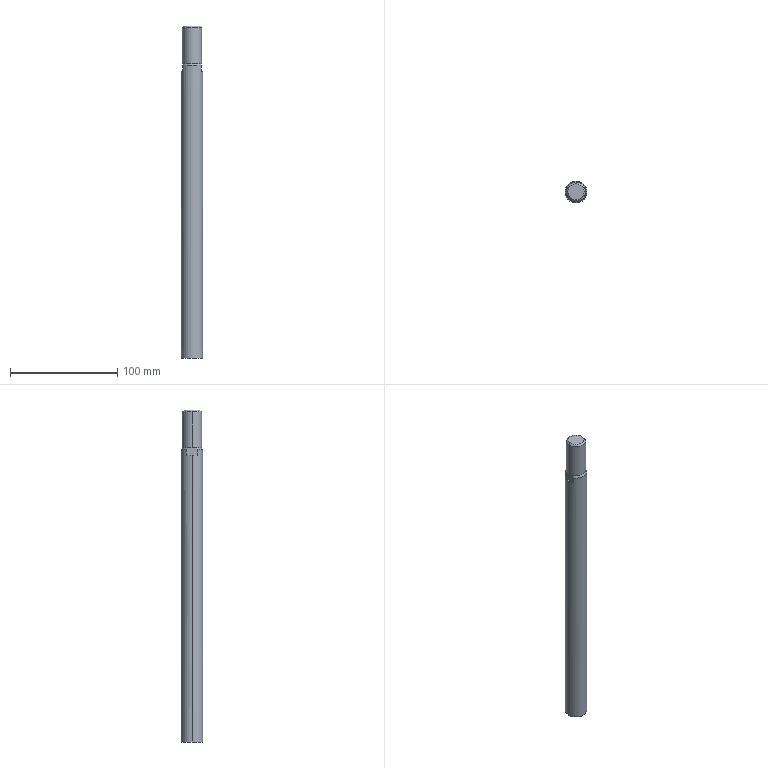Part | STEP file | MDBD50-250-A56 (Rod) | 1 solid | 16 faces | box 20 x 20 x 309 mm | volume 94732 mm3 | cone 4 | cylinder 4 | plane 4 | spline 4 | commonest cylinder face diameters 18 x2 20 x2